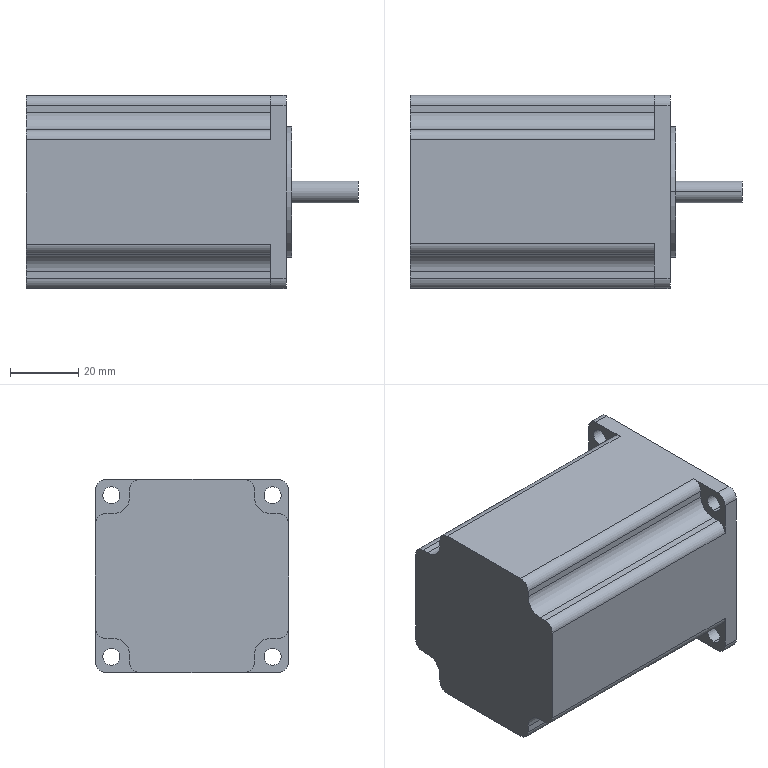Part | SolidWorks | features ICE 4, Fillet 2, CirPattern 1, Extrusion 1 | 1 solid | 48 faces | box 97 x 56.4 x 56.4 mm | volume 215664 mm3 | cylinder 28 | plane 20 | commonest cylinder face diameters 6 x12 5 x8 10 x4 6.35 x2 38.1 x2
STEP:
#1=CARTESIAN_POINT('',(76.,23.55,21.05));
#2=VERTEX_POINT('',#1);
#3=CARTESIAN_POINT('',(76.,23.55,26.05));
#4=VERTEX_POINT('',#3);
#5=CARTESIAN_POINT('',(76.,23.55,23.55));
#6=DIRECTION('',(-1.,0.,0.));
#7=DIRECTION('',(0.,0.,1.));
#8=AXIS2_PLACEMENT_3D('',#5,#6,#7);
#9=CIRCLE('',#8,2.5);
#10=EDGE_CURVE('',#2,#4,#9,.T.);
#11=ORIENTED_EDGE('',*,*,#10,.F.);
#12=CARTESIAN_POINT('',(71.4,23.55,21.05));
#13=VERTEX_POINT('',#12);
#14=CARTESIAN_POINT('',(76.4,23.55,21.05));
#15=DIRECTION('',(-1.,0.,0.));
#16=VECTOR('',#15,1000.);
#17=LINE('',#14,#16);
#18=EDGE_CURVE('',#2,#13,#17,.T.);
#19=ORIENTED_EDGE('',*,*,#18,.T.);
#20=CARTESIAN_POINT('',(71.4,23.55,26.05));
#21=VERTEX_POINT('',#20);
#22=CARTESIAN_POINT('',(71.4,23.55,23.55));
#23=DIRECTION('',(-1.,0.,0.));
#24=DIRECTION('',(0.,-1.,0.));
#25=AXIS2_PLACEMENT_3D('',#22,#23,#24);
#26=CIRCLE('',#25,2.5);
#27=EDGE_CURVE('',#13,#21,#26,.T.);
#28=ORIENTED_EDGE('',*,*,#27,.T.);
#29=CARTESIAN_POINT('',(76.4,23.55,26.05));
#30=DIRECTION('',(-1.,0.,0.));
#31=VECTOR('',#30,1000.);
#32=LINE('',#29,#31);
#33=EDGE_CURVE('',#4,#21,#32,.T.);
#34=ORIENTED_EDGE('',*,*,#33,.F.);
#35=EDGE_LOOP('',(#11,#19,#28,#34));
#36=FACE_OUTER_BOUND('',#35,.T.);
#37=CARTESIAN_POINT('',(76.4,23.55,23.55));
#38=DIRECTION('',(-1.,0.,0.));
#39=DIRECTION('',(0.,0.,1.));
#40=AXIS2_PLACEMENT_3D('',#37,#38,#39);
#41=CYLINDRICAL_SURFACE('',#40,2.5);
#42=ADVANCED_FACE('',(#36),#41,.F.);
#43=CARTESIAN_POINT('',(76.,-23.55,21.05));
#44=VERTEX_POINT('',#43);
#45=CARTESIAN_POINT('',(76.,-23.55,26.05));
#46=VERTEX_POINT('',#45);
#47=CARTESIAN_POINT('',(76.,-23.55,23.55));
#48=DIRECTION('',(-1.,0.,0.));
#49=DIRECTION('',(0.,0.,1.));
#50=AXIS2_PLACEMENT_3D('',#47,#48,#49);
#51=CIRCLE('',#50,2.5);
#52=EDGE_CURVE('',#44,#46,#51,.T.);
#53=ORIENTED_EDGE('',*,*,#52,.F.);
#54=CARTESIAN_POINT('',(71.4,-23.55,21.05));
#55=VERTEX_POINT('',#54);
#56=CARTESIAN_POINT('',(76.4,-23.55,21.05));
#57=DIRECTION('',(-1.,0.,0.));
#58=VECTOR('',#57,1000.);
#59=LINE('',#56,#58);
#60=EDGE_CURVE('',#44,#55,#59,.T.);
#61=ORIENTED_EDGE('',*,*,#60,.T.);
#62=CARTESIAN_POINT('',(71.4,-23.55,26.05));
#63=VERTEX_POINT('',#62);
#64=CARTESIAN_POINT('',(71.4,-23.55,23.55));
#65=DIRECTION('',(-1.,0.,0.));
#66=DIRECTION('',(0.,0.,-1.));
#67=AXIS2_PLACEMENT_3D('',#64,#65,#66);
#68=CIRCLE('',#67,2.5);
#69=EDGE_CURVE('',#55,#63,#68,.T.);
#70=ORIENTED_EDGE('',*,*,#69,.T.);
#71=CARTESIAN_POINT('',(76.4,-23.55,26.05));
#72=DIRECTION('',(-1.,0.,0.));
#73=VECTOR('',#72,1000.);
#74=LINE('',#71,#73);
#75=EDGE_CURVE('',#46,#63,#74,.T.);
#76=ORIENTED_EDGE('',*,*,#75,.F.);
#77=EDGE_LOOP('',(#53,#61,#70,#76));
#78=FACE_OUTER_BOUND('',#77,.T.);
#79=CARTESIAN_POINT('',(76.4,-23.55,23.55));
#80=DIRECTION('',(-1.,0.,0.));
#81=DIRECTION('',(0.,0.,1.));
#82=AXIS2_PLACEMENT_3D('',#79,#80,#81);
#83=CYLINDRICAL_SURFACE('',#82,2.5);
#84=ADVANCED_FACE('',(#78),#83,.F.);
#85=CARTESIAN_POINT('',(76.,-23.55,-26.05));
#86=VERTEX_POINT('',#85);
#87=CARTESIAN_POINT('',(76.,-23.55,-21.05));
#88=VERTEX_POINT('',#87);
#89=CARTESIAN_POINT('',(76.,-23.55,-23.55));
#90=DIRECTION('',(-1.,0.,0.));
#91=DIRECTION('',(0.,0.,1.));
#92=AXIS2_PLACEMENT_3D('',#89,#90,#91);
#93=CIRCLE('',#92,2.5);
#94=EDGE_CURVE('',#86,#88,#93,.T.);
#95=ORIENTED_EDGE('',*,*,#94,.F.);
#96=CARTESIAN_POINT('',(71.4,-23.55,-26.05));
#97=VERTEX_POINT('',#96);
#98=CARTESIAN_POINT('',(76.4,-23.55,-26.05));
#99=DIRECTION('',(-1.,0.,0.));
#100=VECTOR('',#99,1000.);
#101=LINE('',#98,#100);
#102=EDGE_CURVE('',#86,#97,#101,.T.);
#103=ORIENTED_EDGE('',*,*,#102,.T.);
#104=CARTESIAN_POINT('',(71.4,-23.55,-21.05));
#105=VERTEX_POINT('',#104);
#106=CARTESIAN_POINT('',(71.4,-23.55,-23.55));
#107=DIRECTION('',(-1.,0.,0.));
#108=DIRECTION('',(0.,1.,0.));
#109=AXIS2_PLACEMENT_3D('',#106,#107,#108);
#110=CIRCLE('',#109,2.5);
#111=EDGE_CURVE('',#97,#105,#110,.T.);
#112=ORIENTED_EDGE('',*,*,#111,.T.);
#113=CARTESIAN_POINT('',(76.4,-23.55,-21.05));
#114=DIRECTION('',(-1.,0.,0.));
#115=VECTOR('',#114,1000.);
#116=LINE('',#113,#115);
#117=EDGE_CURVE('',#88,#105,#116,.T.);
#118=ORIENTED_EDGE('',*,*,#117,.F.);
#119=EDGE_LOOP('',(#95,#103,#112,#118));
#120=FACE_OUTER_BOUND('',#119,.T.);
#121=CARTESIAN_POINT('',(76.4,-23.55,-23.55));
#122=DIRECTION('',(-1.,0.,0.));
#123=DIRECTION('',(0.,0.,1.));
#124=AXIS2_PLACEMENT_3D('',#121,#122,#123);
#125=CYLINDRICAL_SURFACE('',#124,2.5);
#126=ADVANCED_FACE('',(#120),#125,.F.);
#127=CARTESIAN_POINT('',(76.,23.55,-26.05));
#128=VERTEX_POINT('',#127);
#129=CARTESIAN_POINT('',(76.,23.55,-21.05));
#130=VERTEX_POINT('',#129);
#131=CARTESIAN_POINT('',(76.,23.55,-23.55));
#132=DIRECTION('',(-1.,0.,0.));
#133=DIRECTION('',(0.,0.,1.));
#134=AXIS2_PLACEMENT_3D('',#131,#132,#133);
#135=CIRCLE('',#134,2.5);
#136=EDGE_CURVE('',#128,#130,#135,.T.);
#137=ORIENTED_EDGE('',*,*,#136,.F.);
#138=CARTESIAN_POINT('',(71.4,23.55,-26.05));
#139=VERTEX_POINT('',#138);
#140=CARTESIAN_POINT('',(76.4,23.55,-26.05));
#141=DIRECTION('',(-1.,0.,0.));
#142=VECTOR('',#141,1000.);
#143=LINE('',#140,#142);
#144=EDGE_CURVE('',#128,#139,#143,.T.);
#145=ORIENTED_EDGE('',*,*,#144,.T.);
#146=CARTESIAN_POINT('',(71.4,23.55,-21.05));
#147=VERTEX_POINT('',#146);
#148=CARTESIAN_POINT('',(71.4,23.55,-23.55));
#149=DIRECTION('',(-1.,0.,0.));
#150=DIRECTION('',(0.,0.,1.));
#151=AXIS2_PLACEMENT_3D('',#148,#149,#150);
#152=CIRCLE('',#151,2.5);
#153=EDGE_CURVE('',#139,#147,#152,.T.);
#154=ORIENTED_EDGE('',*,*,#153,.T.);
#155=CARTESIAN_POINT('',(76.4,23.55,-21.05));
#156=DIRECTION('',(-1.,0.,0.));
#157=VECTOR('',#156,1000.);
#158=LINE('',#155,#157);
#159=EDGE_CURVE('',#130,#147,#158,.T.);
#160=ORIENTED_EDGE('',*,*,#159,.F.);
#161=EDGE_LOOP('',(#137,#145,#154,#160));
#162=FACE_OUTER_BOUND('',#161,.T.);
#163=CARTESIAN_POINT('',(76.4,23.55,-23.55));
#164=DIRECTION('',(-1.,0.,0.));
#165=DIRECTION('',(0.,0.,1.));
#166=AXIS2_PLACEMENT_3D('',#163,#164,#165);
#167=CYLINDRICAL_SURFACE('',#166,2.5);
#168=ADVANCED_FACE('',(#162),#167,.F.);
#169=CARTESIAN_POINT('',(97.,0.,-3.175));
#170=VERTEX_POINT('',#169);
#171=CARTESIAN_POINT('',(97.,0.,3.175));
#172=VERTEX_POINT('',#171);
#173=CARTESIAN_POINT('',(97.,0.,0.));
#174=DIRECTION('',(1.,0.,0.));
#175=DIRECTION('',(0.,0.,-1.));
#176=AXIS2_PLACEMENT_3D('',#173,#174,#175);
#177=CIRCLE('',#176,3.175);
#178=EDGE_CURVE('',#170,#172,#177,.T.);
#179=ORIENTED_EDGE('',*,*,#178,.F.);
#180=CARTESIAN_POINT('',(77.6,0.,-3.175));
#181=VERTEX_POINT('',#180);
#182=CARTESIAN_POINT('',(97.,0.,-3.175));
#183=DIRECTION('',(-1.,0.,0.));
#184=VECTOR('',#183,1000.);
#185=LINE('',#182,#184);
#186=EDGE_CURVE('',#170,#181,#185,.T.);
#187=ORIENTED_EDGE('',*,*,#186,.T.);
#188=CARTESIAN_POINT('',(77.6,0.,3.175));
#189=VERTEX_POINT('',#188);
#190=CARTESIAN_POINT('',(77.6,0.,0.));
#191=DIRECTION('',(1.,0.,0.));
#192=DIRECTION('',(0.,0.,-1.));
#193=AXIS2_PLACEMENT_3D('',#190,#191,#192);
#194=CIRCLE('',#193,3.175);
#195=EDGE_CURVE('',#181,#189,#194,.T.);
#196=ORIENTED_EDGE('',*,*,#195,.T.);
#197=CARTESIAN_POINT('',(97.,0.,3.175));
#198=DIRECTION('',(-1.,0.,0.));
#199=VECTOR('',#198,1000.);
#200=LINE('',#197,#199);
#201=EDGE_CURVE('',#172,#189,#200,.T.);
#202=ORIENTED_EDGE('',*,*,#201,.F.);
#203=EDGE_LOOP('',(#179,#187,#196,#202));
#204=FACE_OUTER_BOUND('',#203,.T.);
#205=CARTESIAN_POINT('',(97.,0.,0.));
#206=DIRECTION('',(-1.,0.,0.));
#207=DIRECTION('',(0.,0.,1.));
#208=AXIS2_PLACEMENT_3D('',#205,#206,#207);
#209=CYLINDRICAL_SURFACE('',#208,3.175);
#210=ADVANCED_FACE('',(#204),#209,.T.);
#211=CARTESIAN_POINT('',(77.6,0.,-19.05));
#212=VERTEX_POINT('',#211);
#213=CARTESIAN_POINT('',(77.6,0.,19.05));
#214=VERTEX_POINT('',#213);
#215=CARTESIAN_POINT('',(77.6,0.,0.));
#216=DIRECTION('',(1.,0.,0.));
#217=DIRECTION('',(0.,0.,-1.));
#218=AXIS2_PLACEMENT_3D('',#215,#216,#217);
#219=CIRCLE('',#218,19.05);
#220=EDGE_CURVE('',#212,#214,#219,.T.);
#221=ORIENTED_EDGE('',*,*,#220,.F.);
#222=CARTESIAN_POINT('',(76.,0.,-19.05));
#223=VERTEX_POINT('',#222);
#224=CARTESIAN_POINT('',(77.6,0.,-19.05));
#225=DIRECTION('',(-1.,0.,0.));
#226=VECTOR('',#225,1000.);
#227=LINE('',#224,#226);
#228=EDGE_CURVE('',#212,#223,#227,.T.);
#229=ORIENTED_EDGE('',*,*,#228,.T.);
#230=CARTESIAN_POINT('',(76.,0.,19.05));
#231=VERTEX_POINT('',#230);
#232=CARTESIAN_POINT('',(76.,0.,0.));
#233=DIRECTION('',(1.,0.,0.));
#234=DIRECTION('',(0.,0.,1.));
#235=AXIS2_PLACEMENT_3D('',#232,#233,#234);
#236=CIRCLE('',#235,19.05);
#237=EDGE_CURVE('',#223,#231,#236,.T.);
#238=ORIENTED_EDGE('',*,*,#237,.T.);
#239=CARTESIAN_POINT('',(77.6,0.,19.05));
#240=DIRECTION('',(-1.,0.,0.));
#241=VECTOR('',#240,1000.);
#242=LINE('',#239,#241);
#243=EDGE_CURVE('',#214,#231,#242,.T.);
#244=ORIENTED_EDGE('',*,*,#243,.F.);
#245=EDGE_LOOP('',(#221,#229,#238,#244));
#246=FACE_OUTER_BOUND('',#245,.T.);
#247=CARTESIAN_POINT('',(77.6,0.,0.));
#248=DIRECTION('',(-1.,0.,0.));
#249=DIRECTION('',(0.,0.,1.));
#250=AXIS2_PLACEMENT_3D('',#247,#248,#249);
#251=CYLINDRICAL_SURFACE('',#250,19.05);
#252=ADVANCED_FACE('',(#246),#251,.T.);
#253=CARTESIAN_POINT('',(71.4,28.2,25.2));
#254=VERTEX_POINT('',#253);
#255=CARTESIAN_POINT('',(76.,28.2,25.2));
#256=VERTEX_POINT('',#255);
#257=CARTESIAN_POINT('',(76.,28.2,25.2));
#258=DIRECTION('',(1.,0.,0.));
#259=VECTOR('',#258,1000.);
#260=LINE('',#257,#259);
#261=EDGE_CURVE('',#254,#256,#260,.T.);
#262=ORIENTED_EDGE('',*,*,#261,.F.);
#263=CARTESIAN_POINT('',(71.4,25.2,28.2));
#264=VERTEX_POINT('',#263);
#265=CARTESIAN_POINT('',(71.4,25.2,25.2));
#266=DIRECTION('',(1.,0.,0.));
#267=DIRECTION('',(0.,0.,1.));
#268=AXIS2_PLACEMENT_3D('',#265,#266,#267);
#269=CIRCLE('',#268,3.);
#270=EDGE_CURVE('',#254,#264,#269,.T.);
#271=ORIENTED_EDGE('',*,*,#270,.T.);
#272=CARTESIAN_POINT('',(76.,25.2,28.2));
#273=VERTEX_POINT('',#272);
#274=CARTESIAN_POINT('',(76.,25.2,28.2));
#275=DIRECTION('',(-1.,0.,0.));
#276=VECTOR('',#275,1000.);
#277=LINE('',#274,#276);
#278=EDGE_CURVE('',#273,#264,#277,.T.);
#279=ORIENTED_EDGE('',*,*,#278,.F.);
#280=CARTESIAN_POINT('',(76.,25.2,25.2));
#281=DIRECTION('',(1.,0.,0.));
#282=DIRECTION('',(0.,0.,1.));
#283=AXIS2_PLACEMENT_3D('',#280,#281,#282);
#284=CIRCLE('',#283,3.);
#285=EDGE_CURVE('',#256,#273,#284,.T.);
#286=ORIENTED_EDGE('',*,*,#285,.F.);
#287=EDGE_LOOP('',(#262,#271,#279,#286));
#288=FACE_OUTER_BOUND('',#287,.T.);
#289=CARTESIAN_POINT('',(76.,25.2,25.2));
#290=DIRECTION('',(-1.,0.,0.));
#291=DIRECTION('',(0.,0.,1.));
#292=AXIS2_PLACEMENT_3D('',#289,#290,#291);
#293=CYLINDRICAL_SURFACE('',#292,3.);
#294=ADVANCED_FACE('',(#288),#293,.T.);
#295=CARTESIAN_POINT('',(71.4,-25.2,28.2));
#296=VERTEX_POINT('',#295);
#297=CARTESIAN_POINT('',(76.,-25.2,28.2));
#298=VERTEX_POINT('',#297);
#299=CARTESIAN_POINT('',(76.,-25.2,28.2));
#300=DIRECTION('',(1.,0.,0.));
#301=VECTOR('',#300,1000.);
#302=LINE('',#299,#301);
#303=EDGE_CURVE('',#296,#298,#302,.T.);
#304=ORIENTED_EDGE('',*,*,#303,.F.);
#305=CARTESIAN_POINT('',(71.4,-28.2,25.2));
#306=VERTEX_POINT('',#305);
#307=CARTESIAN_POINT('',(71.4,-25.2,25.2));
#308=DIRECTION('',(1.,0.,0.));
#309=DIRECTION('',(0.,0.,1.));
#310=AXIS2_PLACEMENT_3D('',#307,#308,#309);
#311=CIRCLE('',#310,3.);
#312=EDGE_CURVE('',#296,#306,#311,.T.);
#313=ORIENTED_EDGE('',*,*,#312,.T.);
#314=CARTESIAN_POINT('',(76.,-28.2,25.2));
#315=VERTEX_POINT('',#314);
#316=CARTESIAN_POINT('',(76.,-28.2,25.2));
#317=DIRECTION('',(-1.,0.,0.));
#318=VECTOR('',#317,1000.);
#319=LINE('',#316,#318);
#320=EDGE_CURVE('',#315,#306,#319,.T.);
#321=ORIENTED_EDGE('',*,*,#320,.F.);
#322=CARTESIAN_POINT('',(76.,-25.2,25.2));
#323=DIRECTION('',(1.,0.,0.));
#324=DIRECTION('',(0.,0.,1.));
#325=AXIS2_PLACEMENT_3D('',#322,#323,#324);
#326=CIRCLE('',#325,3.);
#327=EDGE_CURVE('',#298,#315,#326,.T.);
#328=ORIENTED_EDGE('',*,*,#327,.F.);
#329=EDGE_LOOP('',(#304,#313,#321,#328));
#330=FACE_OUTER_BOUND('',#329,.T.);
#331=CARTESIAN_POINT('',(76.,-25.2,25.2));
#332=DIRECTION('',(-1.,0.,0.));
#333=DIRECTION('',(0.,0.,1.));
#334=AXIS2_PLACEMENT_3D('',#331,#332,#333);
#335=CYLINDRICAL_SURFACE('',#334,3.);
#336=ADVANCED_FACE('',(#330),#335,.T.);
#337=CARTESIAN_POINT('',(71.4,-28.2,-25.2));
#338=VERTEX_POINT('',#337);
#339=CARTESIAN_POINT('',(76.,-28.2,-25.2));
#340=VERTEX_POINT('',#339);
#341=CARTESIAN_POINT('',(76.,-28.2,-25.2));
#342=DIRECTION('',(1.,0.,0.));
#343=VECTOR('',#342,1000.);
#344=LINE('',#341,#343);
#345=EDGE_CURVE('',#338,#340,#344,.T.);
#346=ORIENTED_EDGE('',*,*,#345,.F.);
#347=CARTESIAN_POINT('',(71.4,-25.2,-28.2));
#348=VERTEX_POINT('',#347);
#349=CARTESIAN_POINT('',(71.4,-25.2,-25.2));
#350=DIRECTION('',(1.,0.,0.));
#351=DIRECTION('',(0.,0.,1.));
#352=AXIS2_PLACEMENT_3D('',#349,#350,#351);
#353=CIRCLE('',#352,3.);
#354=EDGE_CURVE('',#338,#348,#353,.T.);
#355=ORIENTED_EDGE('',*,*,#354,.T.);
#356=CARTESIAN_POINT('',(76.,-25.2,-28.2));
#357=VERTEX_POINT('',#356);
#358=CARTESIAN_POINT('',(76.,-25.2,-28.2));
#359=DIRECTION('',(-1.,0.,0.));
#360=VECTOR('',#359,1000.);
#361=LINE('',#358,#360);
#362=EDGE_CURVE('',#357,#348,#361,.T.);
#363=ORIENTED_EDGE('',*,*,#362,.F.);
#364=CARTESIAN_POINT('',(76.,-25.2,-25.2));
#365=DIRECTION('',(1.,0.,0.));
#366=DIRECTION('',(0.,0.,1.));
#367=AXIS2_PLACEMENT_3D('',#364,#365,#366);
#368=CIRCLE('',#367,3.);
#369=EDGE_CURVE('',#340,#357,#368,.T.);
#370=ORIENTED_EDGE('',*,*,#369,.F.);
#371=EDGE_LOOP('',(#346,#355,#363,#370));
#372=FACE_OUTER_BOUND('',#371,.T.);
#373=CARTESIAN_POINT('',(76.,-25.2,-25.2));
#374=DIRECTION('',(-1.,0.,0.));
#375=DIRECTION('',(0.,0.,1.));
#376=AXIS2_PLACEMENT_3D('',#373,#374,#375);
#377=CYLINDRICAL_SURFACE('',#376,3.);
#378=ADVANCED_FACE('',(#372),#377,.T.);
#379=CARTESIAN_POINT('',(71.4,25.2,-28.2));
#380=VERTEX_POINT('',#379);
#381=CARTESIAN_POINT('',(76.,25.2,-28.2));
#382=VERTEX_POINT('',#381);
#383=CARTESIAN_POINT('',(76.,25.2,-28.2));
#384=DIRECTION('',(1.,0.,0.));
#385=VECTOR('',#384,1000.);
#386=LINE('',#383,#385);
#387=EDGE_CURVE('',#380,#382,#386,.T.);
#388=ORIENTED_EDGE('',*,*,#387,.F.);
#389=CARTESIAN_POINT('',(71.4,28.2,-25.2));
#390=VERTEX_POINT('',#389);
#391=CARTESIAN_POINT('',(71.4,25.2,-25.2));
#392=DIRECTION('',(1.,0.,0.));
#393=DIRECTION('',(0.,0.,1.));
#394=AXIS2_PLACEMENT_3D('',#391,#392,#393);
#395=CIRCLE('',#394,3.);
#396=EDGE_CURVE('',#380,#390,#395,.T.);
#397=ORIENTED_EDGE('',*,*,#396,.T.);
#398=CARTESIAN_POINT('',(76.,28.2,-25.2));
#399=VERTEX_POINT('',#398);
#400=CARTESIAN_POINT('',(76.,28.2,-25.2));
#401=DIRECTION('',(-1.,0.,0.));
#402=VECTOR('',#401,1000.);
#403=LINE('',#400,#402);
#404=EDGE_CURVE('',#399,#390,#403,.T.);
#405=ORIENTED_EDGE('',*,*,#404,.F.);
#406=CARTESIAN_POINT('',(76.,25.2,-25.2));
#407=DIRECTION('',(1.,0.,0.));
#408=DIRECTION('',(0.,0.,1.));
#409=AXIS2_PLACEMENT_3D('',#406,#407,#408);
#410=CIRCLE('',#409,3.);
#411=EDGE_CURVE('',#382,#399,#410,.T.);
#412=ORIENTED_EDGE('',*,*,#411,.F.);
#413=EDGE_LOOP('',(#388,#397,#405,#412));
#414=FACE_OUTER_BOUND('',#413,.T.);
#415=CARTESIAN_POINT('',(76.,25.2,-25.2));
#416=DIRECTION('',(-1.,0.,0.));
#417=DIRECTION('',(0.,0.,1.));
#418=AXIS2_PLACEMENT_3D('',#415,#416,#417);
#419=CYLINDRICAL_SURFACE('',#418,3.);
#420=ADVANCED_FACE('',(#414),#419,.T.);
#421=CARTESIAN_POINT('',(77.6,0.,0.));
#422=DIRECTION('',(1.,0.,0.));
#423=DIRECTION('',(0.,0.,-1.));
#424=AXIS2_PLACEMENT_3D('',#421,#422,#423);
#425=CIRCLE('',#424,19.05);
#426=EDGE_CURVE('',#214,#212,#425,.T.);
#427=ORIENTED_EDGE('',*,*,#426,.T.);
#428=ORIENTED_EDGE('',*,*,#220,.T.);
#429=EDGE_LOOP('',(#427,#428));
#430=FACE_OUTER_BOUND('',#429,.T.);
#431=CARTESIAN_POINT('',(77.6,0.,0.));
#432=DIRECTION('',(1.,0.,0.));
#433=DIRECTION('',(0.,0.,-1.));
#434=AXIS2_PLACEMENT_3D('',#431,#432,#433);
#435=CIRCLE('',#434,3.175);
#436=EDGE_CURVE('',#189,#181,#435,.T.);
#437=ORIENTED_EDGE('',*,*,#436,.F.);
#438=ORIENTED_EDGE('',*,*,#195,.F.);
#439=EDGE_LOOP('',(#437,#438));
#440=FACE_BOUND('',#439,.T.);
#441=CARTESIAN_POINT('',(77.6,0.,0.));
#442=DIRECTION('',(1.,0.,0.));
#443=DIRECTION('',(0.,0.,-1.));
#444=AXIS2_PLACEMENT_3D('',#441,#442,#443);
#445=PLANE('',#444);
#446=ADVANCED_FACE('',(#430,#440),#445,.T.);
#447=CARTESIAN_POINT('',(76.,23.55,23.55));
#448=DIRECTION('',(-1.,0.,0.));
#449=DIRECTION('',(0.,0.,1.));
#450=AXIS2_PLACEMENT_3D('',#447,#448,#449);
#451=CIRCLE('',#450,2.5);
#452=EDGE_CURVE('',#4,#2,#451,.T.);
#453=ORIENTED_EDGE('',*,*,#452,.T.);
#454=ORIENTED_EDGE('',*,*,#10,.T.);
#455=EDGE_LOOP('',(#453,#454));
#456=FACE_BOUND('',#455,.T.);
#457=CARTESIAN_POINT('',(76.,-23.55,23.55));
#458=DIRECTION('',(-1.,0.,0.));
#459=DIRECTION('',(0.,0.,1.));
#460=AXIS2_PLACEMENT_3D('',#457,#458,#459);
#461=CIRCLE('',#460,2.5);
#462=EDGE_CURVE('',#46,#44,#461,.T.);
#463=ORIENTED_EDGE('',*,*,#462,.T.);
#464=ORIENTED_EDGE('',*,*,#52,.T.);
#465=EDGE_LOOP('',(#463,#464));
#466=FACE_BOUND('',#465,.T.);
#467=CARTESIAN_POINT('',(76.,-23.55,-23.55));
#468=DIRECTION('',(-1.,0.,0.));
#469=DIRECTION('',(0.,0.,1.));
#470=AXIS2_PLACEMENT_3D('',#467,#468,#469);
#471=CIRCLE('',#470,2.5);
#472=EDGE_CURVE('',#88,#86,#471,.T.);
#473=ORIENTED_EDGE('',*,*,#472,.T.);
#474=ORIENTED_EDGE('',*,*,#94,.T.);
#475=EDGE_LOOP('',(#473,#474));
#476=FACE_BOUND('',#475,.T.);
#477=CARTESIAN_POINT('',(76.,23.55,-23.55));
#478=DIRECTION('',(-1.,0.,0.));
#479=DIRECTION('',(0.,0.,1.));
#480=AXIS2_PLACEMENT_3D('',#477,#478,#479);
#481=CIRCLE('',#480,2.5);
#482=EDGE_CURVE('',#130,#128,#481,.T.);
#483=ORIENTED_EDGE('',*,*,#482,.T.);
#484=ORIENTED_EDGE('',*,*,#136,.T.);
#485=EDGE_LOOP('',(#483,#484));
#486=FACE_BOUND('',#485,.T.);
#487=CARTESIAN_POINT('',(76.,-28.2,28.2));
#488=DIRECTION('',(0.,0.,-1.));
#489=VECTOR('',#488,1000.);
#490=LINE('',#487,#489);
#491=EDGE_CURVE('',#315,#340,#490,.T.);
#492=ORIENTED_EDGE('',*,*,#491,.T.);
#493=ORIENTED_EDGE('',*,*,#369,.T.);
#494=CARTESIAN_POINT('',(76.,-28.2,-28.2));
#495=DIRECTION('',(0.,1.,0.));
#496=VECTOR('',#495,1000.);
#497=LINE('',#494,#496);
#498=EDGE_CURVE('',#357,#382,#497,.T.);
#499=ORIENTED_EDGE('',*,*,#498,.T.);
#500=ORIENTED_EDGE('',*,*,#411,.T.);
#501=CARTESIAN_POINT('',(76.,28.2,28.2));
#502=DIRECTION('',(0.,0.,1.));
#503=VECTOR('',#502,1000.);
#504=LINE('',#501,#503);
#505=EDGE_CURVE('',#399,#256,#504,.T.);
#506=ORIENTED_EDGE('',*,*,#505,.T.);
#507=ORIENTED_EDGE('',*,*,#285,.T.);
#508=CARTESIAN_POINT('',(76.,-28.2,28.2));
#509=DIRECTION('',(0.,-1.,0.));
#510=VECTOR('',#509,1000.);
#511=LINE('',#508,#510);
#512=EDGE_CURVE('',#273,#298,#511,.T.);
#513=ORIENTED_EDGE('',*,*,#512,.T.);
#514=ORIENTED_EDGE('',*,*,#327,.T.);
#515=EDGE_LOOP('',(#492,#493,#499,#500,#506,#507,#513,#514));
#516=FACE_OUTER_BOUND('',#515,.T.);
#517=CARTESIAN_POINT('',(76.,0.,0.));
#518=DIRECTION('',(1.,0.,0.));
#519=DIRECTION('',(0.,0.,1.));
#520=AXIS2_PLACEMENT_3D('',#517,#518,#519);
#521=CIRCLE('',#520,19.05);
#522=EDGE_CURVE('',#231,#223,#521,.T.);
#523=ORIENTED_EDGE('',*,*,#522,.F.);
#524=ORIENTED_EDGE('',*,*,#237,.F.);
#525=EDGE_LOOP('',(#523,#524));
#526=FACE_BOUND('',#525,.T.);
#527=CARTESIAN_POINT('',(76.,0.,0.));
#528=DIRECTION('',(-1.,0.,0.));
#529=DIRECTION('',(0.,0.,1.));
#530=AXIS2_PLACEMENT_3D('',#527,#528,#529);
#531=PLANE('',#530);
#532=ADVANCED_FACE('',(#456,#466,#476,#486,#516,#526),#531,.F.);
#533=CARTESIAN_POINT('',(71.4,-15.2,-28.2));
#534=VERTEX_POINT('',#533);
#535=CARTESIAN_POINT('',(71.4,-28.2,-28.2));
#536=DIRECTION('',(0.,1.,0.));
#537=VECTOR('',#536,1000.);
#538=LINE('',#535,#537);
#539=EDGE_CURVE('',#348,#534,#538,.T.);
#540=ORIENTED_EDGE('',*,*,#539,.T.);
#541=CARTESIAN_POINT('',(0.,-15.2,-28.2));
#542=VERTEX_POINT('',#541);
#543=CARTESIAN_POINT('',(76.,-15.2,-28.2));
#544=DIRECTION('',(-1.,0.,0.));
#545=VECTOR('',#544,1000.);
#546=LINE('',#543,#545);
#547=EDGE_CURVE('',#534,#542,#546,.T.);
#548=ORIENTED_EDGE('',*,*,#547,.T.);
#549=CARTESIAN_POINT('',(0.,15.2,-28.2));
#550=VERTEX_POINT('',#549);
#551=CARTESIAN_POINT('',(0.,-28.2,-28.2));
#552=DIRECTION('',(0.,1.,0.));
#553=VECTOR('',#552,1000.);
#554=LINE('',#551,#553);
#555=EDGE_CURVE('',#542,#550,#554,.T.);
#556=ORIENTED_EDGE('',*,*,#555,.T.);
#557=CARTESIAN_POINT('',(71.4,15.2,-28.2));
#558=VERTEX_POINT('',#557);
#559=CARTESIAN_POINT('',(76.,15.2,-28.2));
#560=DIRECTION('',(1.,0.,0.));
#561=VECTOR('',#560,1000.);
#562=LINE('',#559,#561);
#563=EDGE_CURVE('',#550,#558,#562,.T.);
#564=ORIENTED_EDGE('',*,*,#563,.T.);
#565=CARTESIAN_POINT('',(71.4,28.2,-28.2));
#566=DIRECTION('',(0.,1.,0.));
#567=VECTOR('',#566,1000.);
#568=LINE('',#565,#567);
#569=EDGE_CURVE('',#558,#380,#568,.T.);
#570=ORIENTED_EDGE('',*,*,#569,.T.);
#571=ORIENTED_EDGE('',*,*,#387,.T.);
#572=ORIENTED_EDGE('',*,*,#498,.F.);
#573=ORIENTED_EDGE('',*,*,#362,.T.);
#574=EDGE_LOOP('',(#540,#548,#556,#564,#570,#571,#572,#573));
#575=FACE_OUTER_BOUND('',#574,.T.);
#576=CARTESIAN_POINT('',(76.,-28.2,-28.2));
#577=DIRECTION('',(0.,0.,1.));
#578=DIRECTION('',(1.,0.,0.));
#579=AXIS2_PLACEMENT_3D('',#576,#577,#578);
#580=PLANE('',#579);
#581=ADVANCED_FACE('',(#575),#580,.F.);
#582=CARTESIAN_POINT('',(0.,28.2,-15.2));
#583=VERTEX_POINT('',#582);
#584=CARTESIAN_POINT('',(0.,28.2,15.2));
#585=VERTEX_POINT('',#584);
#586=CARTESIAN_POINT('',(0.,28.2,28.2));
#587=DIRECTION('',(0.,0.,1.));
#588=VECTOR('',#587,1000.);
#589=LINE('',#586,#588);
#590=EDGE_CURVE('',#583,#585,#589,.T.);
#591=ORIENTED_EDGE('',*,*,#590,.T.);
#592=CARTESIAN_POINT('',(71.4,28.2,15.2));
#593=VERTEX_POINT('',#592);
#594=CARTESIAN_POINT('',(76.,28.2,15.2));
#595=DIRECTION('',(1.,0.,0.));
#596=VECTOR('',#595,1000.);
#597=LINE('',#594,#596);
#598=EDGE_CURVE('',#585,#593,#597,.T.);
#599=ORIENTED_EDGE('',*,*,#598,.T.);
#600=CARTESIAN_POINT('',(71.4,28.2,28.2));
#601=DIRECTION('',(0.,0.,1.));
#602=VECTOR('',#601,1000.);
#603=LINE('',#600,#602);
#604=EDGE_CURVE('',#593,#254,#603,.T.);
#605=ORIENTED_EDGE('',*,*,#604,.T.);
#606=ORIENTED_EDGE('',*,*,#261,.T.);
#607=ORIENTED_EDGE('',*,*,#505,.F.);
#608=ORIENTED_EDGE('',*,*,#404,.T.);
#609=CARTESIAN_POINT('',(71.4,28.2,-15.2));
#610=VERTEX_POINT('',#609);
#611=CARTESIAN_POINT('',(71.4,28.2,-28.2));
#612=DIRECTION('',(0.,0.,1.));
#613=VECTOR('',#612,1000.);
#614=LINE('',#611,#613);
#615=EDGE_CURVE('',#390,#610,#614,.T.);
#616=ORIENTED_EDGE('',*,*,#615,.T.);
#617=CARTESIAN_POINT('',(76.,28.2,-15.2));
#618=DIRECTION('',(-1.,0.,0.));
#619=VECTOR('',#618,1000.);
#620=LINE('',#617,#619);
#621=EDGE_CURVE('',#610,#583,#620,.T.);
#622=ORIENTED_EDGE('',*,*,#621,.T.);
#623=EDGE_LOOP('',(#591,#599,#605,#606,#607,#608,#616,#622));
#624=FACE_OUTER_BOUND('',#623,.T.);
#625=CARTESIAN_POINT('',(76.,28.2,28.2));
#626=DIRECTION('',(0.,-1.,0.));
#627=DIRECTION('',(0.,0.,-1.));
#628=AXIS2_PLACEMENT_3D('',#625,#626,#627);
#629=PLANE('',#628);
#630=ADVANCED_FACE('',(#624),#629,.F.);
#631=CARTESIAN_POINT('',(71.4,15.2,28.2));
#632=VERTEX_POINT('',#631);
#633=CARTESIAN_POINT('',(71.4,28.2,28.2));
#634=DIRECTION('',(0.,-1.,0.));
#635=VECTOR('',#634,1000.);
#636=LINE('',#633,#635);
#637=EDGE_CURVE('',#264,#632,#636,.T.);
#638=ORIENTED_EDGE('',*,*,#637,.T.);
#639=CARTESIAN_POINT('',(0.,15.2,28.2));
#640=VERTEX_POINT('',#639);
#641=CARTESIAN_POINT('',(76.,15.2,28.2));
#642=DIRECTION('',(-1.,0.,0.));
#643=VECTOR('',#642,1000.);
#644=LINE('',#641,#643);
#645=EDGE_CURVE('',#632,#640,#644,.T.);
#646=ORIENTED_EDGE('',*,*,#645,.T.);
#647=CARTESIAN_POINT('',(0.,-15.2,28.2));
#648=VERTEX_POINT('',#647);
#649=CARTESIAN_POINT('',(0.,-28.2,28.2));
#650=DIRECTION('',(0.,-1.,0.));
#651=VECTOR('',#650,1000.);
#652=LINE('',#649,#651);
#653=EDGE_CURVE('',#640,#648,#652,.T.);
#654=ORIENTED_EDGE('',*,*,#653,.T.);
#655=CARTESIAN_POINT('',(71.4,-15.2,28.2));
#656=VERTEX_POINT('',#655);
#657=CARTESIAN_POINT('',(76.,-15.2,28.2));
#658=DIRECTION('',(1.,0.,0.));
#659=VECTOR('',#658,1000.);
#660=LINE('',#657,#659);
#661=EDGE_CURVE('',#648,#656,#660,.T.);
#662=ORIENTED_EDGE('',*,*,#661,.T.);
#663=CARTESIAN_POINT('',(71.4,-28.2,28.2));
#664=DIRECTION('',(0.,-1.,0.));
#665=VECTOR('',#664,1000.);
#666=LINE('',#663,#665);
#667=EDGE_CURVE('',#656,#296,#666,.T.);
#668=ORIENTED_EDGE('',*,*,#667,.T.);
#669=ORIENTED_EDGE('',*,*,#303,.T.);
#670=ORIENTED_EDGE('',*,*,#512,.F.);
#671=ORIENTED_EDGE('',*,*,#278,.T.);
#672=EDGE_LOOP('',(#638,#646,#654,#662,#668,#669,#670,#671));
#673=FACE_OUTER_BOUND('',#672,.T.);
#674=CARTESIAN_POINT('',(76.,-28.2,28.2));
#675=DIRECTION('',(0.,0.,-1.));
#676=DIRECTION('',(-1.,0.,0.));
#677=AXIS2_PLACEMENT_3D('',#674,#675,#676);
#678=PLANE('',#677);
#679=ADVANCED_FACE('',(#673),#678,.F.);
#680=CARTESIAN_POINT('',(71.4,-28.2,15.2));
#681=VERTEX_POINT('',#680);
#682=CARTESIAN_POINT('',(71.4,-28.2,28.2));
#683=DIRECTION('',(0.,0.,-1.));
#684=VECTOR('',#683,1000.);
#685=LINE('',#682,#684);
#686=EDGE_CURVE('',#306,#681,#685,.T.);
#687=ORIENTED_EDGE('',*,*,#686,.T.);
#688=CARTESIAN_POINT('',(0.,-28.2,15.2));
#689=VERTEX_POINT('',#688);
#690=CARTESIAN_POINT('',(76.,-28.2,15.2));
#691=DIRECTION('',(-1.,0.,0.));
#692=VECTOR('',#691,1000.);
#693=LINE('',#690,#692);
#694=EDGE_CURVE('',#681,#689,#693,.T.);
#695=ORIENTED_EDGE('',*,*,#694,.T.);
#696=CARTESIAN_POINT('',(0.,-28.2,-15.2));
#697=VERTEX_POINT('',#696);
#698=CARTESIAN_POINT('',(0.,-28.2,28.2));
#699=DIRECTION('',(0.,0.,-1.));
#700=VECTOR('',#699,1000.);
#701=LINE('',#698,#700);
#702=EDGE_CURVE('',#689,#697,#701,.T.);
#703=ORIENTED_EDGE('',*,*,#702,.T.);
#704=CARTESIAN_POINT('',(71.4,-28.2,-15.2));
#705=VERTEX_POINT('',#704);
#706=CARTESIAN_POINT('',(76.,-28.2,-15.2));
#707=DIRECTION('',(1.,0.,0.));
#708=VECTOR('',#707,1000.);
#709=LINE('',#706,#708);
#710=EDGE_CURVE('',#697,#705,#709,.T.);
#711=ORIENTED_EDGE('',*,*,#710,.T.);
#712=CARTESIAN_POINT('',(71.4,-28.2,-28.2));
#713=DIRECTION('',(0.,0.,-1.));
#714=VECTOR('',#713,1000.);
#715=LINE('',#712,#714);
#716=EDGE_CURVE('',#705,#338,#715,.T.);
#717=ORIENTED_EDGE('',*,*,#716,.T.);
#718=ORIENTED_EDGE('',*,*,#345,.T.);
#719=ORIENTED_EDGE('',*,*,#491,.F.);
#720=ORIENTED_EDGE('',*,*,#320,.T.);
#721=EDGE_LOOP('',(#687,#695,#703,#711,#717,#718,#719,#720));
#722=FACE_OUTER_BOUND('',#721,.T.);
#723=CARTESIAN_POINT('',(76.,-28.2,28.2));
#724=DIRECTION('',(0.,1.,0.));
#725=DIRECTION('',(0.,0.,1.));
#726=AXIS2_PLACEMENT_3D('',#723,#724,#725);
#727=PLANE('',#726);
#728=ADVANCED_FACE('',(#722),#727,.F.);
#729=ORIENTED_EDGE('',*,*,#653,.F.);
#730=CARTESIAN_POINT('',(0.,18.2,25.2));
#731=VERTEX_POINT('',#730);
#732=CARTESIAN_POINT('',(0.,15.2,25.2));
#733=DIRECTION('',(-1.,0.,0.));
#734=DIRECTION('',(0.,0.,1.));
#735=AXIS2_PLACEMENT_3D('',#732,#733,#734);
#736=CIRCLE('',#735,3.);
#737=EDGE_CURVE('',#640,#731,#736,.T.);
#738=ORIENTED_EDGE('',*,*,#737,.T.);
#739=CARTESIAN_POINT('',(0.,18.2,23.2));
#740=VERTEX_POINT('',#739);
#741=CARTESIAN_POINT('',(0.,18.2,28.2));
#742=DIRECTION('',(0.,0.,1.));
#743=VECTOR('',#742,1000.);
#744=LINE('',#741,#743);
#745=EDGE_CURVE('',#740,#731,#744,.T.);
#746=ORIENTED_EDGE('',*,*,#745,.F.);
#747=CARTESIAN_POINT('',(0.,23.2,18.2));
#748=VERTEX_POINT('',#747);
#749=CARTESIAN_POINT('',(0.,23.2,23.2));
#750=DIRECTION('',(-1.,0.,0.));
#751=DIRECTION('',(0.,1.,0.));
#752=AXIS2_PLACEMENT_3D('',#749,#750,#751);
#753=CIRCLE('',#752,5.);
#754=EDGE_CURVE('',#748,#740,#753,.T.);
#755=ORIENTED_EDGE('',*,*,#754,.F.);
#756=CARTESIAN_POINT('',(0.,25.2,18.2));
#757=VERTEX_POINT('',#756);
#758=CARTESIAN_POINT('',(0.,28.2,18.2));
#759=DIRECTION('',(0.,-1.,0.));
#760=VECTOR('',#759,1000.);
#761=LINE('',#758,#760);
#762=EDGE_CURVE('',#757,#748,#761,.T.);
#763=ORIENTED_EDGE('',*,*,#762,.F.);
#764=CARTESIAN_POINT('',(0.,25.2,15.2));
#765=DIRECTION('',(-1.,0.,0.));
#766=DIRECTION('',(0.,0.,1.));
#767=AXIS2_PLACEMENT_3D('',#764,#765,#766);
#768=CIRCLE('',#767,3.);
#769=EDGE_CURVE('',#757,#585,#768,.T.);
#770=ORIENTED_EDGE('',*,*,#769,.T.);
#771=ORIENTED_EDGE('',*,*,#590,.F.);
#772=CARTESIAN_POINT('',(0.,25.2,-18.2));
#773=VERTEX_POINT('',#772);
#774=CARTESIAN_POINT('',(0.,25.2,-15.2));
#775=DIRECTION('',(-1.,0.,0.));
#776=DIRECTION('',(0.,0.,1.));
#777=AXIS2_PLACEMENT_3D('',#774,#775,#776);
#778=CIRCLE('',#777,3.);
#779=EDGE_CURVE('',#583,#773,#778,.T.);
#780=ORIENTED_EDGE('',*,*,#779,.T.);
#781=CARTESIAN_POINT('',(0.,23.2,-18.2));
#782=VERTEX_POINT('',#781);
#783=CARTESIAN_POINT('',(0.,28.2,-18.2));
#784=DIRECTION('',(0.,1.,0.));
#785=VECTOR('',#784,1000.);
#786=LINE('',#783,#785);
#787=EDGE_CURVE('',#782,#773,#786,.T.);
#788=ORIENTED_EDGE('',*,*,#787,.F.);
#789=CARTESIAN_POINT('',(0.,18.2,-23.2));
#790=VERTEX_POINT('',#789);
#791=CARTESIAN_POINT('',(0.,23.2,-23.2));
#792=DIRECTION('',(-1.,0.,0.));
#793=DIRECTION('',(0.,0.,-1.));
#794=AXIS2_PLACEMENT_3D('',#791,#792,#793);
#795=CIRCLE('',#794,5.);
#796=EDGE_CURVE('',#790,#782,#795,.T.);
#797=ORIENTED_EDGE('',*,*,#796,.F.);
#798=CARTESIAN_POINT('',(0.,18.2,-25.2));
#799=VERTEX_POINT('',#798);
#800=CARTESIAN_POINT('',(0.,18.2,-28.2));
#801=DIRECTION('',(0.,0.,1.));
#802=VECTOR('',#801,1000.);
#803=LINE('',#800,#802);
#804=EDGE_CURVE('',#799,#790,#803,.T.);
#805=ORIENTED_EDGE('',*,*,#804,.F.);
#806=CARTESIAN_POINT('',(0.,15.2,-25.2));
#807=DIRECTION('',(-1.,0.,0.));
#808=DIRECTION('',(0.,0.,1.));
#809=AXIS2_PLACEMENT_3D('',#806,#807,#808);
#810=CIRCLE('',#809,3.);
#811=EDGE_CURVE('',#799,#550,#810,.T.);
#812=ORIENTED_EDGE('',*,*,#811,.T.);
#813=ORIENTED_EDGE('',*,*,#555,.F.);
#814=CARTESIAN_POINT('',(0.,-18.2,-25.2));
#815=VERTEX_POINT('',#814);
#816=CARTESIAN_POINT('',(0.,-15.2,-25.2));
#817=DIRECTION('',(-1.,0.,0.));
#818=DIRECTION('',(0.,0.,1.));
#819=AXIS2_PLACEMENT_3D('',#816,#817,#818);
#820=CIRCLE('',#819,3.);
#821=EDGE_CURVE('',#542,#815,#820,.T.);
#822=ORIENTED_EDGE('',*,*,#821,.T.);
#823=CARTESIAN_POINT('',(0.,-18.2,-23.2));
#824=VERTEX_POINT('',#823);
#825=CARTESIAN_POINT('',(0.,-18.2,-28.2));
#826=DIRECTION('',(0.,0.,-1.));
#827=VECTOR('',#826,1000.);
#828=LINE('',#825,#827);
#829=EDGE_CURVE('',#824,#815,#828,.T.);
#830=ORIENTED_EDGE('',*,*,#829,.F.);
#831=CARTESIAN_POINT('',(0.,-23.2,-18.2));
#832=VERTEX_POINT('',#831);
#833=CARTESIAN_POINT('',(0.,-23.2,-23.2));
#834=DIRECTION('',(-1.,0.,0.));
#835=DIRECTION('',(0.,-1.,0.));
#836=AXIS2_PLACEMENT_3D('',#833,#834,#835);
#837=CIRCLE('',#836,5.);
#838=EDGE_CURVE('',#832,#824,#837,.T.);
#839=ORIENTED_EDGE('',*,*,#838,.F.);
#840=CARTESIAN_POINT('',(0.,-25.2,-18.2));
#841=VERTEX_POINT('',#840);
#842=CARTESIAN_POINT('',(0.,-28.2,-18.2));
#843=DIRECTION('',(0.,1.,0.));
#844=VECTOR('',#843,1000.);
#845=LINE('',#842,#844);
#846=EDGE_CURVE('',#841,#832,#845,.T.);
#847=ORIENTED_EDGE('',*,*,#846,.F.);
#848=CARTESIAN_POINT('',(0.,-25.2,-15.2));
#849=DIRECTION('',(-1.,0.,0.));
#850=DIRECTION('',(0.,0.,1.));
#851=AXIS2_PLACEMENT_3D('',#848,#849,#850);
#852=CIRCLE('',#851,3.);
#853=EDGE_CURVE('',#841,#697,#852,.T.);
#854=ORIENTED_EDGE('',*,*,#853,.T.);
#855=ORIENTED_EDGE('',*,*,#702,.F.);
#856=CARTESIAN_POINT('',(0.,-25.2,18.2));
#857=VERTEX_POINT('',#856);
#858=CARTESIAN_POINT('',(0.,-25.2,15.2));
#859=DIRECTION('',(-1.,0.,0.));
#860=DIRECTION('',(0.,0.,1.));
#861=AXIS2_PLACEMENT_3D('',#858,#859,#860);
#862=CIRCLE('',#861,3.);
#863=EDGE_CURVE('',#689,#857,#862,.T.);
#864=ORIENTED_EDGE('',*,*,#863,.T.);
#865=CARTESIAN_POINT('',(0.,-23.2,18.2));
#866=VERTEX_POINT('',#865);
#867=CARTESIAN_POINT('',(0.,-28.2,18.2));
#868=DIRECTION('',(0.,-1.,0.));
#869=VECTOR('',#868,1000.);
#870=LINE('',#867,#869);
#871=EDGE_CURVE('',#866,#857,#870,.T.);
#872=ORIENTED_EDGE('',*,*,#871,.F.);
#873=CARTESIAN_POINT('',(0.,-18.2,23.2));
#874=VERTEX_POINT('',#873);
#875=CARTESIAN_POINT('',(0.,-23.2,23.2));
#876=DIRECTION('',(-1.,0.,0.));
#877=DIRECTION('',(0.,0.,1.));
#878=AXIS2_PLACEMENT_3D('',#875,#876,#877);
#879=CIRCLE('',#878,5.);
#880=EDGE_CURVE('',#874,#866,#879,.T.);
#881=ORIENTED_EDGE('',*,*,#880,.F.);
#882=CARTESIAN_POINT('',(0.,-18.2,25.2));
#883=VERTEX_POINT('',#882);
#884=CARTESIAN_POINT('',(0.,-18.2,28.2));
#885=DIRECTION('',(0.,0.,-1.));
#886=VECTOR('',#885,1000.);
#887=LINE('',#884,#886);
#888=EDGE_CURVE('',#883,#874,#887,.T.);
#889=ORIENTED_EDGE('',*,*,#888,.F.);
#890=CARTESIAN_POINT('',(0.,-15.2,25.2));
#891=DIRECTION('',(-1.,0.,0.));
#892=DIRECTION('',(0.,0.,1.));
#893=AXIS2_PLACEMENT_3D('',#890,#891,#892);
#894=CIRCLE('',#893,3.);
#895=EDGE_CURVE('',#883,#648,#894,.T.);
#896=ORIENTED_EDGE('',*,*,#895,.T.);
#897=EDGE_LOOP('',(#729,#738,#746,#755,#763,#770,#771,#780,#788,#797,#805,#812,#813,#822,#830,#839,#847,#854,#855,#864,#872,#881,#889,#896));
#898=FACE_OUTER_BOUND('',#897,.T.);
#899=CARTESIAN_POINT('',(0.,0.,0.));
#900=DIRECTION('',(-1.,0.,0.));
#901=DIRECTION('',(0.,0.,1.));
#902=AXIS2_PLACEMENT_3D('',#899,#900,#901);
#903=PLANE('',#902);
#904=ADVANCED_FACE('',(#898),#903,.T.);
#905=ORIENTED_EDGE('',*,*,#228,.F.);
#906=ORIENTED_EDGE('',*,*,#426,.F.);
#907=ORIENTED_EDGE('',*,*,#243,.T.);
#908=ORIENTED_EDGE('',*,*,#522,.T.);
#909=EDGE_LOOP('',(#905,#906,#907,#908));
#910=FACE_OUTER_BOUND('',#909,.T.);
#911=CARTESIAN_POINT('',(77.6,0.,0.));
#912=DIRECTION('',(-1.,0.,0.));
#913=DIRECTION('',(0.,0.,1.));
#914=AXIS2_PLACEMENT_3D('',#911,#912,#913);
#915=CYLINDRICAL_SURFACE('',#914,19.05);
#916=ADVANCED_FACE('',(#910),#915,.T.);
#917=ORIENTED_EDGE('',*,*,#186,.F.);
#918=CARTESIAN_POINT('',(97.,0.,0.));
#919=DIRECTION('',(1.,0.,0.));
#920=DIRECTION('',(0.,0.,-1.));
#921=AXIS2_PLACEMENT_3D('',#918,#919,#920);
#922=CIRCLE('',#921,3.175);
#923=EDGE_CURVE('',#172,#170,#922,.T.);
#924=ORIENTED_EDGE('',*,*,#923,.F.);
#925=ORIENTED_EDGE('',*,*,#201,.T.);
#926=ORIENTED_EDGE('',*,*,#436,.T.);
#927=EDGE_LOOP('',(#917,#924,#925,#926));
#928=FACE_OUTER_BOUND('',#927,.T.);
#929=CARTESIAN_POINT('',(97.,0.,0.));
#930=DIRECTION('',(-1.,0.,0.));
#931=DIRECTION('',(0.,0.,1.));
#932=AXIS2_PLACEMENT_3D('',#929,#930,#931);
#933=CYLINDRICAL_SURFACE('',#932,3.175);
#934=ADVANCED_FACE('',(#928),#933,.T.);
#935=ORIENTED_EDGE('',*,*,#923,.T.);
#936=ORIENTED_EDGE('',*,*,#178,.T.);
#937=EDGE_LOOP('',(#935,#936));
#938=FACE_OUTER_BOUND('',#937,.T.);
#939=CARTESIAN_POINT('',(97.,0.,0.));
#940=DIRECTION('',(1.,0.,0.));
#941=DIRECTION('',(0.,0.,-1.));
#942=AXIS2_PLACEMENT_3D('',#939,#940,#941);
#943=PLANE('',#942);
#944=ADVANCED_FACE('',(#938),#943,.T.);
#945=ORIENTED_EDGE('',*,*,#787,.T.);
#946=CARTESIAN_POINT('',(71.4,25.2,-18.2));
#947=VERTEX_POINT('',#946);
#948=CARTESIAN_POINT('',(90.142,25.2,-18.2));
#949=DIRECTION('',(1.,0.,0.));
#950=VECTOR('',#949,1000.);
#951=LINE('',#948,#950);
#952=EDGE_CURVE('',#773,#947,#951,.T.);
#953=ORIENTED_EDGE('',*,*,#952,.T.);
#954=CARTESIAN_POINT('',(71.4,23.2,-18.2));
#955=VERTEX_POINT('',#954);
#956=CARTESIAN_POINT('',(71.4,28.2,-18.2));
#957=DIRECTION('',(0.,-1.,0.));
#958=VECTOR('',#957,1000.);
#959=LINE('',#956,#958);
#960=EDGE_CURVE('',#947,#955,#959,.T.);
#961=ORIENTED_EDGE('',*,*,#960,.T.);
#962=CARTESIAN_POINT('',(90.142,23.2,-18.2));
#963=DIRECTION('',(-1.,0.,0.));
#964=VECTOR('',#963,1000.);
#965=LINE('',#962,#964);
#966=EDGE_CURVE('',#955,#782,#965,.T.);
#967=ORIENTED_EDGE('',*,*,#966,.T.);
#968=EDGE_LOOP('',(#945,#953,#961,#967));
#969=FACE_OUTER_BOUND('',#968,.T.);
#970=CARTESIAN_POINT('',(90.142,28.2,-18.2));
#971=DIRECTION('',(0.,0.,1.));
#972=DIRECTION('',(1.,0.,0.));
#973=AXIS2_PLACEMENT_3D('',#970,#971,#972);
#974=PLANE('',#973);
#975=ADVANCED_FACE('',(#969),#974,.F.);
#976=CARTESIAN_POINT('',(71.4,18.2,-23.2));
#977=VERTEX_POINT('',#976);
#978=CARTESIAN_POINT('',(71.4,23.2,-23.2));
#979=DIRECTION('',(1.,0.,0.));
#980=DIRECTION('',(0.,0.,1.));
#981=AXIS2_PLACEMENT_3D('',#978,#979,#980);
#982=CIRCLE('',#981,5.);
#983=EDGE_CURVE('',#955,#977,#982,.T.);
#984=ORIENTED_EDGE('',*,*,#983,.T.);
#985=CARTESIAN_POINT('',(90.142,18.2,-23.2));
#986=DIRECTION('',(-1.,0.,0.));
#987=VECTOR('',#986,1000.);
#988=LINE('',#985,#987);
#989=EDGE_CURVE('',#977,#790,#988,.T.);
#990=ORIENTED_EDGE('',*,*,#989,.T.);
#991=ORIENTED_EDGE('',*,*,#796,.T.);
#992=ORIENTED_EDGE('',*,*,#966,.F.);
#993=EDGE_LOOP('',(#984,#990,#991,#992));
#994=FACE_OUTER_BOUND('',#993,.T.);
#995=CARTESIAN_POINT('',(90.142,23.2,-23.2));
#996=DIRECTION('',(-1.,0.,0.));
#997=DIRECTION('',(0.,0.,1.));
#998=AXIS2_PLACEMENT_3D('',#995,#996,#997);
#999=CYLINDRICAL_SURFACE('',#998,5.);
#1000=ADVANCED_FACE('',(#994),#999,.F.);
#1001=CARTESIAN_POINT('',(71.4,18.2,-25.2));
#1002=VERTEX_POINT('',#1001);
#1003=CARTESIAN_POINT('',(71.4,18.2,-28.2));
#1004=DIRECTION('',(0.,0.,-1.));
#1005=VECTOR('',#1004,1000.);
#1006=LINE('',#1003,#1005);
#1007=EDGE_CURVE('',#977,#1002,#1006,.T.);
#1008=ORIENTED_EDGE('',*,*,#1007,.T.);
#1009=CARTESIAN_POINT('',(90.142,18.2,-25.2));
#1010=DIRECTION('',(-1.,0.,0.));
#1011=VECTOR('',#1010,1000.);
#1012=LINE('',#1009,#1011);
#1013=EDGE_CURVE('',#1002,#799,#1012,.T.);
#1014=ORIENTED_EDGE('',*,*,#1013,.T.);
#1015=ORIENTED_EDGE('',*,*,#804,.T.);
#1016=ORIENTED_EDGE('',*,*,#989,.F.);
#1017=EDGE_LOOP('',(#1008,#1014,#1015,#1016));
#1018=FACE_OUTER_BOUND('',#1017,.T.);
#1019=CARTESIAN_POINT('',(90.142,18.2,-28.2));
#1020=DIRECTION('',(0.,-1.,0.));
#1021=DIRECTION('',(0.,0.,-1.));
#1022=AXIS2_PLACEMENT_3D('',#1019,#1020,#1021);
#1023=PLANE('',#1022);
#1024=ADVANCED_FACE('',(#1018),#1023,.F.);
#1025=CARTESIAN_POINT('',(71.4,23.55,-23.55));
#1026=DIRECTION('',(-1.,0.,0.));
#1027=DIRECTION('',(0.,0.,1.));
#1028=AXIS2_PLACEMENT_3D('',#1025,#1026,#1027);
#1029=CIRCLE('',#1028,2.5);
#1030=EDGE_CURVE('',#147,#139,#1029,.T.);
#1031=ORIENTED_EDGE('',*,*,#1030,.F.);
#1032=ORIENTED_EDGE('',*,*,#153,.F.);
#1033=EDGE_LOOP('',(#1031,#1032));
#1034=FACE_BOUND('',#1033,.T.);
#1035=ORIENTED_EDGE('',*,*,#569,.F.);
#1036=CARTESIAN_POINT('',(71.4,15.2,-25.2));
#1037=DIRECTION('',(1.,0.,0.));
#1038=DIRECTION('',(0.,0.,1.));
#1039=AXIS2_PLACEMENT_3D('',#1036,#1037,#1038);
#1040=CIRCLE('',#1039,3.);
#1041=EDGE_CURVE('',#558,#1002,#1040,.T.);
#1042=ORIENTED_EDGE('',*,*,#1041,.T.);
#1043=ORIENTED_EDGE('',*,*,#1007,.F.);
#1044=ORIENTED_EDGE('',*,*,#983,.F.);
#1045=ORIENTED_EDGE('',*,*,#960,.F.);
#1046=CARTESIAN_POINT('',(71.4,25.2,-15.2));
#1047=DIRECTION('',(1.,0.,0.));
#1048=DIRECTION('',(0.,0.,1.));
#1049=AXIS2_PLACEMENT_3D('',#1046,#1047,#1048);
#1050=CIRCLE('',#1049,3.);
#1051=EDGE_CURVE('',#947,#610,#1050,.T.);
#1052=ORIENTED_EDGE('',*,*,#1051,.T.);
#1053=ORIENTED_EDGE('',*,*,#615,.F.);
#1054=ORIENTED_EDGE('',*,*,#396,.F.);
#1055=EDGE_LOOP('',(#1035,#1042,#1043,#1044,#1045,#1052,#1053,#1054));
#1056=FACE_OUTER_BOUND('',#1055,.T.);
#1057=CARTESIAN_POINT('',(71.4,0.,0.));
#1058=DIRECTION('',(-1.,0.,0.));
#1059=DIRECTION('',(0.,0.,1.));
#1060=AXIS2_PLACEMENT_3D('',#1057,#1058,#1059);
#1061=PLANE('',#1060);
#1062=ADVANCED_FACE('',(#1034,#1056),#1061,.T.);
#1063=ORIENTED_EDGE('',*,*,#144,.F.);
#1064=ORIENTED_EDGE('',*,*,#482,.F.);
#1065=ORIENTED_EDGE('',*,*,#159,.T.);
#1066=ORIENTED_EDGE('',*,*,#1030,.T.);
#1067=EDGE_LOOP('',(#1063,#1064,#1065,#1066));
#1068=FACE_OUTER_BOUND('',#1067,.T.);
#1069=CARTESIAN_POINT('',(76.4,23.55,-23.55));
#1070=DIRECTION('',(-1.,0.,0.));
#1071=DIRECTION('',(0.,0.,1.));
#1072=AXIS2_PLACEMENT_3D('',#1069,#1070,#1071);
#1073=CYLINDRICAL_SURFACE('',#1072,2.5);
#1074=ADVANCED_FACE('',(#1068),#1073,.F.);
#1075=ORIENTED_EDGE('',*,*,#829,.T.);
#1076=CARTESIAN_POINT('',(71.4,-18.2,-25.2));
#1077=VERTEX_POINT('',#1076);
#1078=CARTESIAN_POINT('',(90.142,-18.2,-25.2));
#1079=DIRECTION('',(1.,0.,0.));
#1080=VECTOR('',#1079,1000.);
#1081=LINE('',#1078,#1080);
#1082=EDGE_CURVE('',#815,#1077,#1081,.T.);
#1083=ORIENTED_EDGE('',*,*,#1082,.T.);
#1084=CARTESIAN_POINT('',(71.4,-18.2,-23.2));
#1085=VERTEX_POINT('',#1084);
#1086=CARTESIAN_POINT('',(71.4,-18.2,-28.2));
#1087=DIRECTION('',(0.,0.,1.));
#1088=VECTOR('',#1087,1000.);
#1089=LINE('',#1086,#1088);
#1090=EDGE_CURVE('',#1077,#1085,#1089,.T.);
#1091=ORIENTED_EDGE('',*,*,#1090,.T.);
#1092=CARTESIAN_POINT('',(90.142,-18.2,-23.2));
#1093=DIRECTION('',(-1.,0.,0.));
#1094=VECTOR('',#1093,1000.);
#1095=LINE('',#1092,#1094);
#1096=EDGE_CURVE('',#1085,#824,#1095,.T.);
#1097=ORIENTED_EDGE('',*,*,#1096,.T.);
#1098=EDGE_LOOP('',(#1075,#1083,#1091,#1097));
#1099=FACE_OUTER_BOUND('',#1098,.T.);
#1100=CARTESIAN_POINT('',(90.142,-18.2,-28.2));
#1101=DIRECTION('',(0.,1.,0.));
#1102=DIRECTION('',(0.,0.,1.));
#1103=AXIS2_PLACEMENT_3D('',#1100,#1101,#1102);
#1104=PLANE('',#1103);
#1105=ADVANCED_FACE('',(#1099),#1104,.F.);
#1106=CARTESIAN_POINT('',(71.4,-23.2,-18.2));
#1107=VERTEX_POINT('',#1106);
#1108=CARTESIAN_POINT('',(71.4,-23.2,-23.2));
#1109=DIRECTION('',(1.,0.,0.));
#1110=DIRECTION('',(0.,0.,1.));
#1111=AXIS2_PLACEMENT_3D('',#1108,#1109,#1110);
#1112=CIRCLE('',#1111,5.);
#1113=EDGE_CURVE('',#1085,#1107,#1112,.T.);
#1114=ORIENTED_EDGE('',*,*,#1113,.T.);
#1115=CARTESIAN_POINT('',(90.142,-23.2,-18.2));
#1116=DIRECTION('',(-1.,0.,0.));
#1117=VECTOR('',#1116,1000.);
#1118=LINE('',#1115,#1117);
#1119=EDGE_CURVE('',#1107,#832,#1118,.T.);
#1120=ORIENTED_EDGE('',*,*,#1119,.T.);
#1121=ORIENTED_EDGE('',*,*,#838,.T.);
#1122=ORIENTED_EDGE('',*,*,#1096,.F.);
#1123=EDGE_LOOP('',(#1114,#1120,#1121,#1122));
#1124=FACE_OUTER_BOUND('',#1123,.T.);
#1125=CARTESIAN_POINT('',(90.142,-23.2,-23.2));
#1126=DIRECTION('',(-1.,0.,0.));
#1127=DIRECTION('',(0.,0.,1.));
#1128=AXIS2_PLACEMENT_3D('',#1125,#1126,#1127);
#1129=CYLINDRICAL_SURFACE('',#1128,5.);
#1130=ADVANCED_FACE('',(#1124),#1129,.F.);
#1131=CARTESIAN_POINT('',(71.4,-25.2,-18.2));
#1132=VERTEX_POINT('',#1131);
#1133=CARTESIAN_POINT('',(71.4,-28.2,-18.2));
#1134=DIRECTION('',(0.,-1.,0.));
#1135=VECTOR('',#1134,1000.);
#1136=LINE('',#1133,#1135);
#1137=EDGE_CURVE('',#1107,#1132,#1136,.T.);
#1138=ORIENTED_EDGE('',*,*,#1137,.T.);
#1139=CARTESIAN_POINT('',(90.142,-25.2,-18.2));
#1140=DIRECTION('',(-1.,0.,0.));
#1141=VECTOR('',#1140,1000.);
#1142=LINE('',#1139,#1141);
#1143=EDGE_CURVE('',#1132,#841,#1142,.T.);
#1144=ORIENTED_EDGE('',*,*,#1143,.T.);
#1145=ORIENTED_EDGE('',*,*,#846,.T.);
#1146=ORIENTED_EDGE('',*,*,#1119,.F.);
#1147=EDGE_LOOP('',(#1138,#1144,#1145,#1146));
#1148=FACE_OUTER_BOUND('',#1147,.T.);
#1149=CARTESIAN_POINT('',(90.142,-28.2,-18.2));
#1150=DIRECTION('',(0.,0.,1.));
#1151=DIRECTION('',(0.,-1.,0.));
#1152=AXIS2_PLACEMENT_3D('',#1149,#1150,#1151);
#1153=PLANE('',#1152);
#1154=ADVANCED_FACE('',(#1148),#1153,.F.);
#1155=CARTESIAN_POINT('',(71.4,-23.55,-23.55));
#1156=DIRECTION('',(-1.,0.,0.));
#1157=DIRECTION('',(0.,1.,0.));
#1158=AXIS2_PLACEMENT_3D('',#1155,#1156,#1157);
#1159=CIRCLE('',#1158,2.5);
#1160=EDGE_CURVE('',#105,#97,#1159,.T.);
#1161=ORIENTED_EDGE('',*,*,#1160,.F.);
#1162=ORIENTED_EDGE('',*,*,#111,.F.);
#1163=EDGE_LOOP('',(#1161,#1162));
#1164=FACE_BOUND('',#1163,.T.);
#1165=ORIENTED_EDGE('',*,*,#716,.F.);
#1166=CARTESIAN_POINT('',(71.4,-25.2,-15.2));
#1167=DIRECTION('',(1.,0.,0.));
#1168=DIRECTION('',(0.,0.,1.));
#1169=AXIS2_PLACEMENT_3D('',#1166,#1167,#1168);
#1170=CIRCLE('',#1169,3.);
#1171=EDGE_CURVE('',#705,#1132,#1170,.T.);
#1172=ORIENTED_EDGE('',*,*,#1171,.T.);
#1173=ORIENTED_EDGE('',*,*,#1137,.F.);
#1174=ORIENTED_EDGE('',*,*,#1113,.F.);
#1175=ORIENTED_EDGE('',*,*,#1090,.F.);
#1176=CARTESIAN_POINT('',(71.4,-15.2,-25.2));
#1177=DIRECTION('',(1.,0.,0.));
#1178=DIRECTION('',(0.,0.,1.));
#1179=AXIS2_PLACEMENT_3D('',#1176,#1177,#1178);
#1180=CIRCLE('',#1179,3.);
#1181=EDGE_CURVE('',#1077,#534,#1180,.T.);
#1182=ORIENTED_EDGE('',*,*,#1181,.T.);
#1183=ORIENTED_EDGE('',*,*,#539,.F.);
#1184=ORIENTED_EDGE('',*,*,#354,.F.);
#1185=EDGE_LOOP('',(#1165,#1172,#1173,#1174,#1175,#1182,#1183,#1184));
#1186=FACE_OUTER_BOUND('',#1185,.T.);
#1187=CARTESIAN_POINT('',(71.4,0.,0.));
#1188=DIRECTION('',(-1.,0.,0.));
#1189=DIRECTION('',(0.,0.,1.));
#1190=AXIS2_PLACEMENT_3D('',#1187,#1188,#1189);
#1191=PLANE('',#1190);
#1192=ADVANCED_FACE('',(#1164,#1186),#1191,.T.);
#1193=ORIENTED_EDGE('',*,*,#871,.T.);
#1194=CARTESIAN_POINT('',(71.4,-25.2,18.2));
#1195=VERTEX_POINT('',#1194);
#1196=CARTESIAN_POINT('',(90.142,-25.2,18.2));
#1197=DIRECTION('',(1.,0.,0.));
#1198=VECTOR('',#1197,1000.);
#1199=LINE('',#1196,#1198);
#1200=EDGE_CURVE('',#857,#1195,#1199,.T.);
#1201=ORIENTED_EDGE('',*,*,#1200,.T.);
#1202=CARTESIAN_POINT('',(71.4,-23.2,18.2));
#1203=VERTEX_POINT('',#1202);
#1204=CARTESIAN_POINT('',(71.4,-28.2,18.2));
#1205=DIRECTION('',(0.,1.,0.));
#1206=VECTOR('',#1205,1000.);
#1207=LINE('',#1204,#1206);
#1208=EDGE_CURVE('',#1195,#1203,#1207,.T.);
#1209=ORIENTED_EDGE('',*,*,#1208,.T.);
#1210=CARTESIAN_POINT('',(90.142,-23.2,18.2));
#1211=DIRECTION('',(-1.,0.,0.));
#1212=VECTOR('',#1211,1000.);
#1213=LINE('',#1210,#1212);
#1214=EDGE_CURVE('',#1203,#866,#1213,.T.);
#1215=ORIENTED_EDGE('',*,*,#1214,.T.);
#1216=EDGE_LOOP('',(#1193,#1201,#1209,#1215));
#1217=FACE_OUTER_BOUND('',#1216,.T.);
#1218=CARTESIAN_POINT('',(90.142,-28.2,18.2));
#1219=DIRECTION('',(0.,0.,-1.));
#1220=DIRECTION('',(-1.,0.,0.));
#1221=AXIS2_PLACEMENT_3D('',#1218,#1219,#1220);
#1222=PLANE('',#1221);
#1223=ADVANCED_FACE('',(#1217),#1222,.F.);
#1224=CARTESIAN_POINT('',(71.4,-18.2,23.2));
#1225=VERTEX_POINT('',#1224);
#1226=CARTESIAN_POINT('',(71.4,-23.2,23.2));
#1227=DIRECTION('',(1.,0.,0.));
#1228=DIRECTION('',(0.,0.,1.));
#1229=AXIS2_PLACEMENT_3D('',#1226,#1227,#1228);
#1230=CIRCLE('',#1229,5.);
#1231=EDGE_CURVE('',#1203,#1225,#1230,.T.);
#1232=ORIENTED_EDGE('',*,*,#1231,.T.);
#1233=CARTESIAN_POINT('',(90.142,-18.2,23.2));
#1234=DIRECTION('',(-1.,0.,0.));
#1235=VECTOR('',#1234,1000.);
#1236=LINE('',#1233,#1235);
#1237=EDGE_CURVE('',#1225,#874,#1236,.T.);
#1238=ORIENTED_EDGE('',*,*,#1237,.T.);
#1239=ORIENTED_EDGE('',*,*,#880,.T.);
#1240=ORIENTED_EDGE('',*,*,#1214,.F.);
#1241=EDGE_LOOP('',(#1232,#1238,#1239,#1240));
#1242=FACE_OUTER_BOUND('',#1241,.T.);
#1243=CARTESIAN_POINT('',(90.142,-23.2,23.2));
#1244=DIRECTION('',(-1.,0.,0.));
#1245=DIRECTION('',(0.,0.,1.));
#1246=AXIS2_PLACEMENT_3D('',#1243,#1244,#1245);
#1247=CYLINDRICAL_SURFACE('',#1246,5.);
#1248=ADVANCED_FACE('',(#1242),#1247,.F.);
#1249=CARTESIAN_POINT('',(71.4,-18.2,25.2));
#1250=VERTEX_POINT('',#1249);
#1251=CARTESIAN_POINT('',(71.4,-18.2,28.2));
#1252=DIRECTION('',(0.,0.,1.));
#1253=VECTOR('',#1252,1000.);
#1254=LINE('',#1251,#1253);
#1255=EDGE_CURVE('',#1225,#1250,#1254,.T.);
#1256=ORIENTED_EDGE('',*,*,#1255,.T.);
#1257=CARTESIAN_POINT('',(90.142,-18.2,25.2));
#1258=DIRECTION('',(-1.,0.,0.));
#1259=VECTOR('',#1258,1000.);
#1260=LINE('',#1257,#1259);
#1261=EDGE_CURVE('',#1250,#883,#1260,.T.);
#1262=ORIENTED_EDGE('',*,*,#1261,.T.);
#1263=ORIENTED_EDGE('',*,*,#888,.T.);
#1264=ORIENTED_EDGE('',*,*,#1237,.F.);
#1265=EDGE_LOOP('',(#1256,#1262,#1263,#1264));
#1266=FACE_OUTER_BOUND('',#1265,.T.);
#1267=CARTESIAN_POINT('',(90.142,-18.2,28.2));
#1268=DIRECTION('',(0.,1.,0.));
#1269=DIRECTION('',(0.,0.,1.));
#1270=AXIS2_PLACEMENT_3D('',#1267,#1268,#1269);
#1271=PLANE('',#1270);
#1272=ADVANCED_FACE('',(#1266),#1271,.F.);
#1273=CARTESIAN_POINT('',(71.4,-23.55,23.55));
#1274=DIRECTION('',(-1.,0.,0.));
#1275=DIRECTION('',(0.,0.,-1.));
#1276=AXIS2_PLACEMENT_3D('',#1273,#1274,#1275);
#1277=CIRCLE('',#1276,2.5);
#1278=EDGE_CURVE('',#63,#55,#1277,.T.);
#1279=ORIENTED_EDGE('',*,*,#1278,.F.);
#1280=ORIENTED_EDGE('',*,*,#69,.F.);
#1281=EDGE_LOOP('',(#1279,#1280));
#1282=FACE_BOUND('',#1281,.T.);
#1283=ORIENTED_EDGE('',*,*,#667,.F.);
#1284=CARTESIAN_POINT('',(71.4,-15.2,25.2));
#1285=DIRECTION('',(1.,0.,0.));
#1286=DIRECTION('',(0.,0.,1.));
#1287=AXIS2_PLACEMENT_3D('',#1284,#1285,#1286);
#1288=CIRCLE('',#1287,3.);
#1289=EDGE_CURVE('',#656,#1250,#1288,.T.);
#1290=ORIENTED_EDGE('',*,*,#1289,.T.);
#1291=ORIENTED_EDGE('',*,*,#1255,.F.);
#1292=ORIENTED_EDGE('',*,*,#1231,.F.);
#1293=ORIENTED_EDGE('',*,*,#1208,.F.);
#1294=CARTESIAN_POINT('',(71.4,-25.2,15.2));
#1295=DIRECTION('',(1.,0.,0.));
#1296=DIRECTION('',(0.,0.,1.));
#1297=AXIS2_PLACEMENT_3D('',#1294,#1295,#1296);
#1298=CIRCLE('',#1297,3.);
#1299=EDGE_CURVE('',#1195,#681,#1298,.T.);
#1300=ORIENTED_EDGE('',*,*,#1299,.T.);
#1301=ORIENTED_EDGE('',*,*,#686,.F.);
#1302=ORIENTED_EDGE('',*,*,#312,.F.);
#1303=EDGE_LOOP('',(#1283,#1290,#1291,#1292,#1293,#1300,#1301,#1302));
#1304=FACE_OUTER_BOUND('',#1303,.T.);
#1305=CARTESIAN_POINT('',(71.4,0.,0.));
#1306=DIRECTION('',(-1.,0.,0.));
#1307=DIRECTION('',(0.,0.,1.));
#1308=AXIS2_PLACEMENT_3D('',#1305,#1306,#1307);
#1309=PLANE('',#1308);
#1310=ADVANCED_FACE('',(#1282,#1304),#1309,.T.);
#1311=ORIENTED_EDGE('',*,*,#745,.T.);
#1312=CARTESIAN_POINT('',(71.4,18.2,25.2));
#1313=VERTEX_POINT('',#1312);
#1314=CARTESIAN_POINT('',(90.142,18.2,25.2));
#1315=DIRECTION('',(1.,0.,0.));
#1316=VECTOR('',#1315,1000.);
#1317=LINE('',#1314,#1316);
#1318=EDGE_CURVE('',#731,#1313,#1317,.T.);
#1319=ORIENTED_EDGE('',*,*,#1318,.T.);
#1320=CARTESIAN_POINT('',(71.4,18.2,23.2));
#1321=VERTEX_POINT('',#1320);
#1322=CARTESIAN_POINT('',(71.4,18.2,28.2));
#1323=DIRECTION('',(0.,0.,-1.));
#1324=VECTOR('',#1323,1000.);
#1325=LINE('',#1322,#1324);
#1326=EDGE_CURVE('',#1313,#1321,#1325,.T.);
#1327=ORIENTED_EDGE('',*,*,#1326,.T.);
#1328=CARTESIAN_POINT('',(90.142,18.2,23.2));
#1329=DIRECTION('',(-1.,0.,0.));
#1330=VECTOR('',#1329,1000.);
#1331=LINE('',#1328,#1330);
#1332=EDGE_CURVE('',#1321,#740,#1331,.T.);
#1333=ORIENTED_EDGE('',*,*,#1332,.T.);
#1334=EDGE_LOOP('',(#1311,#1319,#1327,#1333));
#1335=FACE_OUTER_BOUND('',#1334,.T.);
#1336=CARTESIAN_POINT('',(90.142,18.2,28.2));
#1337=DIRECTION('',(0.,-1.,0.));
#1338=DIRECTION('',(0.,0.,-1.));
#1339=AXIS2_PLACEMENT_3D('',#1336,#1337,#1338);
#1340=PLANE('',#1339);
#1341=ADVANCED_FACE('',(#1335),#1340,.F.);
#1342=CARTESIAN_POINT('',(71.4,23.2,18.2));
#1343=VERTEX_POINT('',#1342);
#1344=CARTESIAN_POINT('',(71.4,23.2,23.2));
#1345=DIRECTION('',(1.,0.,0.));
#1346=DIRECTION('',(0.,0.,1.));
#1347=AXIS2_PLACEMENT_3D('',#1344,#1345,#1346);
#1348=CIRCLE('',#1347,5.);
#1349=EDGE_CURVE('',#1321,#1343,#1348,.T.);
#1350=ORIENTED_EDGE('',*,*,#1349,.T.);
#1351=CARTESIAN_POINT('',(90.142,23.2,18.2));
#1352=DIRECTION('',(-1.,0.,0.));
#1353=VECTOR('',#1352,1000.);
#1354=LINE('',#1351,#1353);
#1355=EDGE_CURVE('',#1343,#748,#1354,.T.);
#1356=ORIENTED_EDGE('',*,*,#1355,.T.);
#1357=ORIENTED_EDGE('',*,*,#754,.T.);
#1358=ORIENTED_EDGE('',*,*,#1332,.F.);
#1359=EDGE_LOOP('',(#1350,#1356,#1357,#1358));
#1360=FACE_OUTER_BOUND('',#1359,.T.);
#1361=CARTESIAN_POINT('',(90.142,23.2,23.2));
#1362=DIRECTION('',(-1.,0.,0.));
#1363=DIRECTION('',(0.,0.,1.));
#1364=AXIS2_PLACEMENT_3D('',#1361,#1362,#1363);
#1365=CYLINDRICAL_SURFACE('',#1364,5.);
#1366=ADVANCED_FACE('',(#1360),#1365,.F.);
#1367=CARTESIAN_POINT('',(71.4,25.2,18.2));
#1368=VERTEX_POINT('',#1367);
#1369=CARTESIAN_POINT('',(71.4,28.2,18.2));
#1370=DIRECTION('',(0.,1.,0.));
#1371=VECTOR('',#1370,1000.);
#1372=LINE('',#1369,#1371);
#1373=EDGE_CURVE('',#1343,#1368,#1372,.T.);
#1374=ORIENTED_EDGE('',*,*,#1373,.T.);
#1375=CARTESIAN_POINT('',(90.142,25.2,18.2));
#1376=DIRECTION('',(-1.,0.,0.));
#1377=VECTOR('',#1376,1000.);
#1378=LINE('',#1375,#1377);
#1379=EDGE_CURVE('',#1368,#757,#1378,.T.);
#1380=ORIENTED_EDGE('',*,*,#1379,.T.);
#1381=ORIENTED_EDGE('',*,*,#762,.T.);
#1382=ORIENTED_EDGE('',*,*,#1355,.F.);
#1383=EDGE_LOOP('',(#1374,#1380,#1381,#1382));
#1384=FACE_OUTER_BOUND('',#1383,.T.);
#1385=CARTESIAN_POINT('',(90.142,28.2,18.2));
#1386=DIRECTION('',(0.,0.,-1.));
#1387=DIRECTION('',(0.,1.,0.));
#1388=AXIS2_PLACEMENT_3D('',#1385,#1386,#1387);
#1389=PLANE('',#1388);
#1390=ADVANCED_FACE('',(#1384),#1389,.F.);
#1391=CARTESIAN_POINT('',(71.4,23.55,23.55));
#1392=DIRECTION('',(-1.,0.,0.));
#1393=DIRECTION('',(0.,-1.,0.));
#1394=AXIS2_PLACEMENT_3D('',#1391,#1392,#1393);
#1395=CIRCLE('',#1394,2.5);
#1396=EDGE_CURVE('',#21,#13,#1395,.T.);
#1397=ORIENTED_EDGE('',*,*,#1396,.F.);
#1398=ORIENTED_EDGE('',*,*,#27,.F.);
#1399=EDGE_LOOP('',(#1397,#1398));
#1400=FACE_BOUND('',#1399,.T.);
#1401=ORIENTED_EDGE('',*,*,#604,.F.);
#1402=CARTESIAN_POINT('',(71.4,25.2,15.2));
#1403=DIRECTION('',(1.,0.,0.));
#1404=DIRECTION('',(0.,0.,1.));
#1405=AXIS2_PLACEMENT_3D('',#1402,#1403,#1404);
#1406=CIRCLE('',#1405,3.);
#1407=EDGE_CURVE('',#593,#1368,#1406,.T.);
#1408=ORIENTED_EDGE('',*,*,#1407,.T.);
#1409=ORIENTED_EDGE('',*,*,#1373,.F.);
#1410=ORIENTED_EDGE('',*,*,#1349,.F.);
#1411=ORIENTED_EDGE('',*,*,#1326,.F.);
#1412=CARTESIAN_POINT('',(71.4,15.2,25.2));
#1413=DIRECTION('',(1.,0.,0.));
#1414=DIRECTION('',(0.,0.,1.));
#1415=AXIS2_PLACEMENT_3D('',#1412,#1413,#1414);
#1416=CIRCLE('',#1415,3.);
#1417=EDGE_CURVE('',#1313,#632,#1416,.T.);
#1418=ORIENTED_EDGE('',*,*,#1417,.T.);
#1419=ORIENTED_EDGE('',*,*,#637,.F.);
#1420=ORIENTED_EDGE('',*,*,#270,.F.);
#1421=EDGE_LOOP('',(#1401,#1408,#1409,#1410,#1411,#1418,#1419,#1420));
#1422=FACE_OUTER_BOUND('',#1421,.T.);
#1423=CARTESIAN_POINT('',(71.4,0.,0.));
#1424=DIRECTION('',(-1.,0.,0.));
#1425=DIRECTION('',(0.,0.,1.));
#1426=AXIS2_PLACEMENT_3D('',#1423,#1424,#1425);
#1427=PLANE('',#1426);
#1428=ADVANCED_FACE('',(#1400,#1422),#1427,.T.);
#1429=ORIENTED_EDGE('',*,*,#102,.F.);
#1430=ORIENTED_EDGE('',*,*,#472,.F.);
#1431=ORIENTED_EDGE('',*,*,#117,.T.);
#1432=ORIENTED_EDGE('',*,*,#1160,.T.);
#1433=EDGE_LOOP('',(#1429,#1430,#1431,#1432));
#1434=FACE_OUTER_BOUND('',#1433,.T.);
#1435=CARTESIAN_POINT('',(76.4,-23.55,-23.55));
#1436=DIRECTION('',(-1.,0.,0.));
#1437=DIRECTION('',(0.,0.,1.));
#1438=AXIS2_PLACEMENT_3D('',#1435,#1436,#1437);
#1439=CYLINDRICAL_SURFACE('',#1438,2.5);
#1440=ADVANCED_FACE('',(#1434),#1439,.F.);
#1441=ORIENTED_EDGE('',*,*,#60,.F.);
#1442=ORIENTED_EDGE('',*,*,#462,.F.);
#1443=ORIENTED_EDGE('',*,*,#75,.T.);
#1444=ORIENTED_EDGE('',*,*,#1278,.T.);
#1445=EDGE_LOOP('',(#1441,#1442,#1443,#1444));
#1446=FACE_OUTER_BOUND('',#1445,.T.);
#1447=CARTESIAN_POINT('',(76.4,-23.55,23.55));
#1448=DIRECTION('',(-1.,0.,0.));
#1449=DIRECTION('',(0.,0.,1.));
#1450=AXIS2_PLACEMENT_3D('',#1447,#1448,#1449);
#1451=CYLINDRICAL_SURFACE('',#1450,2.5);
#1452=ADVANCED_FACE('',(#1446),#1451,.F.);
#1453=ORIENTED_EDGE('',*,*,#18,.F.);
#1454=ORIENTED_EDGE('',*,*,#452,.F.);
#1455=ORIENTED_EDGE('',*,*,#33,.T.);
#1456=ORIENTED_EDGE('',*,*,#1396,.T.);
#1457=EDGE_LOOP('',(#1453,#1454,#1455,#1456));
#1458=FACE_OUTER_BOUND('',#1457,.T.);
#1459=CARTESIAN_POINT('',(76.4,23.55,23.55));
#1460=DIRECTION('',(-1.,0.,0.));
#1461=DIRECTION('',(0.,0.,1.));
#1462=AXIS2_PLACEMENT_3D('',#1459,#1460,#1461);
#1463=CYLINDRICAL_SURFACE('',#1462,2.5);
#1464=ADVANCED_FACE('',(#1458),#1463,.F.);
#1465=ORIENTED_EDGE('',*,*,#1417,.F.);
#1466=ORIENTED_EDGE('',*,*,#1318,.F.);
#1467=ORIENTED_EDGE('',*,*,#737,.F.);
#1468=ORIENTED_EDGE('',*,*,#645,.F.);
#1469=EDGE_LOOP('',(#1465,#1466,#1467,#1468));
#1470=FACE_OUTER_BOUND('',#1469,.T.);
#1471=CARTESIAN_POINT('',(76.,15.2,25.2));
#1472=DIRECTION('',(-1.,0.,0.));
#1473=DIRECTION('',(0.,0.,1.));
#1474=AXIS2_PLACEMENT_3D('',#1471,#1472,#1473);
#1475=CYLINDRICAL_SURFACE('',#1474,3.);
#1476=ADVANCED_FACE('',(#1470),#1475,.T.);
#1477=ORIENTED_EDGE('',*,*,#1407,.F.);
#1478=ORIENTED_EDGE('',*,*,#598,.F.);
#1479=ORIENTED_EDGE('',*,*,#769,.F.);
#1480=ORIENTED_EDGE('',*,*,#1379,.F.);
#1481=EDGE_LOOP('',(#1477,#1478,#1479,#1480));
#1482=FACE_OUTER_BOUND('',#1481,.T.);
#1483=CARTESIAN_POINT('',(90.142,25.2,15.2));
#1484=DIRECTION('',(-1.,0.,0.));
#1485=DIRECTION('',(0.,0.,1.));
#1486=AXIS2_PLACEMENT_3D('',#1483,#1484,#1485);
#1487=CYLINDRICAL_SURFACE('',#1486,3.);
#1488=ADVANCED_FACE('',(#1482),#1487,.T.);
#1489=ORIENTED_EDGE('',*,*,#1289,.F.);
#1490=ORIENTED_EDGE('',*,*,#661,.F.);
#1491=ORIENTED_EDGE('',*,*,#895,.F.);
#1492=ORIENTED_EDGE('',*,*,#1261,.F.);
#1493=EDGE_LOOP('',(#1489,#1490,#1491,#1492));
#1494=FACE_OUTER_BOUND('',#1493,.T.);
#1495=CARTESIAN_POINT('',(90.142,-15.2,25.2));
#1496=DIRECTION('',(-1.,0.,0.));
#1497=DIRECTION('',(0.,0.,1.));
#1498=AXIS2_PLACEMENT_3D('',#1495,#1496,#1497);
#1499=CYLINDRICAL_SURFACE('',#1498,3.);
#1500=ADVANCED_FACE('',(#1494),#1499,.T.);
#1501=ORIENTED_EDGE('',*,*,#1299,.F.);
#1502=ORIENTED_EDGE('',*,*,#1200,.F.);
#1503=ORIENTED_EDGE('',*,*,#863,.F.);
#1504=ORIENTED_EDGE('',*,*,#694,.F.);
#1505=EDGE_LOOP('',(#1501,#1502,#1503,#1504));
#1506=FACE_OUTER_BOUND('',#1505,.T.);
#1507=CARTESIAN_POINT('',(76.,-25.2,15.2));
#1508=DIRECTION('',(-1.,0.,0.));
#1509=DIRECTION('',(0.,0.,1.));
#1510=AXIS2_PLACEMENT_3D('',#1507,#1508,#1509);
#1511=CYLINDRICAL_SURFACE('',#1510,3.);
#1512=ADVANCED_FACE('',(#1506),#1511,.T.);
#1513=ORIENTED_EDGE('',*,*,#1171,.F.);
#1514=ORIENTED_EDGE('',*,*,#710,.F.);
#1515=ORIENTED_EDGE('',*,*,#853,.F.);
#1516=ORIENTED_EDGE('',*,*,#1143,.F.);
#1517=EDGE_LOOP('',(#1513,#1514,#1515,#1516));
#1518=FACE_OUTER_BOUND('',#1517,.T.);
#1519=CARTESIAN_POINT('',(90.142,-25.2,-15.2));
#1520=DIRECTION('',(-1.,0.,0.));
#1521=DIRECTION('',(0.,0.,1.));
#1522=AXIS2_PLACEMENT_3D('',#1519,#1520,#1521);
#1523=CYLINDRICAL_SURFACE('',#1522,3.);
#1524=ADVANCED_FACE('',(#1518),#1523,.T.);
#1525=ORIENTED_EDGE('',*,*,#1181,.F.);
#1526=ORIENTED_EDGE('',*,*,#1082,.F.);
#1527=ORIENTED_EDGE('',*,*,#821,.F.);
#1528=ORIENTED_EDGE('',*,*,#547,.F.);
#1529=EDGE_LOOP('',(#1525,#1526,#1527,#1528));
#1530=FACE_OUTER_BOUND('',#1529,.T.);
#1531=CARTESIAN_POINT('',(76.,-15.2,-25.2));
#1532=DIRECTION('',(-1.,0.,0.));
#1533=DIRECTION('',(0.,0.,1.));
#1534=AXIS2_PLACEMENT_3D('',#1531,#1532,#1533);
#1535=CYLINDRICAL_SURFACE('',#1534,3.);
#1536=ADVANCED_FACE('',(#1530),#1535,.T.);
#1537=ORIENTED_EDGE('',*,*,#1041,.F.);
#1538=ORIENTED_EDGE('',*,*,#563,.F.);
#1539=ORIENTED_EDGE('',*,*,#811,.F.);
#1540=ORIENTED_EDGE('',*,*,#1013,.F.);
#1541=EDGE_LOOP('',(#1537,#1538,#1539,#1540));
#1542=FACE_OUTER_BOUND('',#1541,.T.);
#1543=CARTESIAN_POINT('',(90.142,15.2,-25.2));
#1544=DIRECTION('',(-1.,0.,0.));
#1545=DIRECTION('',(0.,0.,1.));
#1546=AXIS2_PLACEMENT_3D('',#1543,#1544,#1545);
#1547=CYLINDRICAL_SURFACE('',#1546,3.);
#1548=ADVANCED_FACE('',(#1542),#1547,.T.);
#1549=ORIENTED_EDGE('',*,*,#1051,.F.);
#1550=ORIENTED_EDGE('',*,*,#952,.F.);
#1551=ORIENTED_EDGE('',*,*,#779,.F.);
#1552=ORIENTED_EDGE('',*,*,#621,.F.);
#1553=EDGE_LOOP('',(#1549,#1550,#1551,#1552));
#1554=FACE_OUTER_BOUND('',#1553,.T.);
#1555=CARTESIAN_POINT('',(76.,25.2,-15.2));
#1556=DIRECTION('',(-1.,0.,0.));
#1557=DIRECTION('',(0.,0.,1.));
#1558=AXIS2_PLACEMENT_3D('',#1555,#1556,#1557);
#1559=CYLINDRICAL_SURFACE('',#1558,3.);
#1560=ADVANCED_FACE('',(#1554),#1559,.T.);
#1561=CLOSED_SHELL('',(#42,#84,#126,#168,#210,#252,#294,#336,#378,#420,#446,#532,#581,#630,#679,#728,#904,#916,#934,#944,#975,#1000,#1024,#1062,#1074,#1105,#1130,#1154,#1192,#1223,#1248,#1272,#1310,#1341,#1366,#1390,#1428,#1440,#1452,#1464,#1476,#1488,#1500,#1512,#1524,#1536,#1548,#1560));
#1562=MANIFOLD_SOLID_BREP('',#1561);
#1563=CARTESIAN_POINT('',(0.,0.,0.));
#1564=DIRECTION('',(0.,0.,1.));
#1565=DIRECTION('',(1.,0.,0.));
#1566=AXIS2_PLACEMENT_3D('',#1563,#1564,#1565);
#1567=(LENGTH_UNIT()NAMED_UNIT(*)SI_UNIT(.MILLI.,.METRE.));
#1568=UNCERTAINTY_MEASURE_WITH_UNIT(LENGTH_MEASURE(0.00001),#1567,'','');
#1569=(NAMED_UNIT(*)PLANE_ANGLE_UNIT()SI_UNIT($,.RADIAN.));
#1570=(NAMED_UNIT(*)SI_UNIT($,.STERADIAN.)SOLID_ANGLE_UNIT());
#1571=(GEOMETRIC_REPRESENTATION_CONTEXT(3)GLOBAL_UNCERTAINTY_ASSIGNED_CONTEXT((#1568))GLOBAL_UNIT_ASSIGNED_CONTEXT((#1567,#1569,#1570))REPRESENTATION_CONTEXT('',''));
#1572=ADVANCED_BREP_SHAPE_REPRESENTATION('',(#1562,#1566),#1571);